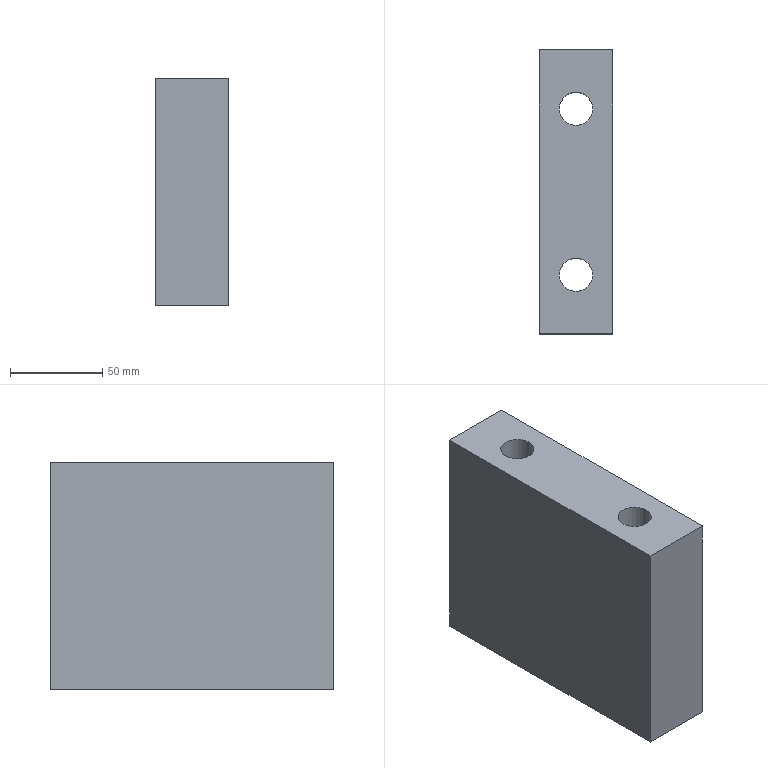Part | NX | features LIN_SOLID_COLOR 2 | 1 solid | 12 faces | box 40 x 154 x 123.5 mm | volume 638424 mm3 | plane 8 | cylinder 4 | commonest cylinder face diameters 18 x2 27 x2
STEP:
#1=CARTESIAN_POINT('',(716.,-77.,-106.5));
#2=VERTEX_POINT('',#1);
#3=CARTESIAN_POINT('',(676.,-77.,-106.5));
#4=VERTEX_POINT('',#3);
#5=CARTESIAN_POINT('',(676.,-77.,-106.5));
#6=DIRECTION('',(-1.,0.,0.));
#7=VECTOR('',#6,1000.);
#8=LINE('',#5,#7);
#9=EDGE_CURVE('',#2,#4,#8,.T.);
#10=ORIENTED_EDGE('',*,*,#9,.T.);
#11=CARTESIAN_POINT('',(676.,-77.,-230.));
#12=VERTEX_POINT('',#11);
#13=CARTESIAN_POINT('',(676.,-77.,-101.5));
#14=DIRECTION('',(0.,0.,1.));
#15=VECTOR('',#14,1000.);
#16=LINE('',#13,#15);
#17=EDGE_CURVE('',#12,#4,#16,.T.);
#18=ORIENTED_EDGE('',*,*,#17,.F.);
#19=CARTESIAN_POINT('',(716.,-77.,-230.));
#20=VERTEX_POINT('',#19);
#21=CARTESIAN_POINT('',(426.,-77.,-230.));
#22=DIRECTION('',(-1.,0.,0.));
#23=VECTOR('',#22,1000.);
#24=LINE('',#21,#23);
#25=EDGE_CURVE('',#20,#12,#24,.T.);
#26=ORIENTED_EDGE('',*,*,#25,.F.);
#27=CARTESIAN_POINT('',(716.,-77.,-101.5));
#28=DIRECTION('',(0.,0.,1.));
#29=VECTOR('',#28,1000.);
#30=LINE('',#27,#29);
#31=EDGE_CURVE('',#20,#2,#30,.T.);
#32=ORIENTED_EDGE('',*,*,#31,.T.);
#33=EDGE_LOOP('',(#10,#18,#26,#32));
#34=FACE_BOUND('',#33,.T.);
#35=CARTESIAN_POINT('',(676.,-77.,-101.5));
#36=DIRECTION('',(0.,1.,0.));
#37=DIRECTION('',(0.,0.,1.));
#38=AXIS2_PLACEMENT_3D('',#35,#36,#37);
#39=PLANE('',#38);
#40=ADVANCED_FACE('',(#34),#39,.F.);
#41=CARTESIAN_POINT('',(676.,77.,-106.5));
#42=VERTEX_POINT('',#41);
#43=CARTESIAN_POINT('',(676.,-160.,-106.5));
#44=DIRECTION('',(0.,-1.,0.));
#45=VECTOR('',#44,1000.);
#46=LINE('',#43,#45);
#47=EDGE_CURVE('',#42,#4,#46,.T.);
#48=ORIENTED_EDGE('',*,*,#47,.F.);
#49=CARTESIAN_POINT('',(676.,77.,-230.));
#50=VERTEX_POINT('',#49);
#51=CARTESIAN_POINT('',(676.,77.,-101.5));
#52=DIRECTION('',(0.,0.,-1.));
#53=VECTOR('',#52,1000.);
#54=LINE('',#51,#53);
#55=EDGE_CURVE('',#50,#42,#54,.F.);
#56=ORIENTED_EDGE('',*,*,#55,.F.);
#57=CARTESIAN_POINT('',(676.,0.,-230.));
#58=DIRECTION('',(0.,1.,0.));
#59=VECTOR('',#58,1000.);
#60=LINE('',#57,#59);
#61=EDGE_CURVE('',#12,#50,#60,.T.);
#62=ORIENTED_EDGE('',*,*,#61,.F.);
#63=ORIENTED_EDGE('',*,*,#17,.T.);
#64=EDGE_LOOP('',(#48,#56,#62,#63));
#65=FACE_BOUND('',#64,.T.);
#66=CARTESIAN_POINT('',(676.,-160.,-101.5));
#67=DIRECTION('',(1.,0.,0.));
#68=DIRECTION('',(0.,0.,1.));
#69=AXIS2_PLACEMENT_3D('',#66,#67,#68);
#70=PLANE('',#69);
#71=ADVANCED_FACE('',(#65),#70,.F.);
#72=CARTESIAN_POINT('',(716.,77.,-230.));
#73=VERTEX_POINT('',#72);
#74=CARTESIAN_POINT('',(716.,77.,-106.5));
#75=VERTEX_POINT('',#74);
#76=CARTESIAN_POINT('',(716.,77.,-101.5));
#77=DIRECTION('',(0.,0.,-1.));
#78=VECTOR('',#77,1000.);
#79=LINE('',#76,#78);
#80=EDGE_CURVE('',#73,#75,#79,.F.);
#81=ORIENTED_EDGE('',*,*,#80,.T.);
#82=CARTESIAN_POINT('',(716.,-160.,-106.5));
#83=DIRECTION('',(0.,-1.,0.));
#84=VECTOR('',#83,1000.);
#85=LINE('',#82,#84);
#86=EDGE_CURVE('',#75,#2,#85,.T.);
#87=ORIENTED_EDGE('',*,*,#86,.T.);
#88=ORIENTED_EDGE('',*,*,#31,.F.);
#89=CARTESIAN_POINT('',(716.,0.,-230.));
#90=DIRECTION('',(0.,1.,0.));
#91=VECTOR('',#90,1000.);
#92=LINE('',#89,#91);
#93=EDGE_CURVE('',#20,#73,#92,.T.);
#94=ORIENTED_EDGE('',*,*,#93,.T.);
#95=EDGE_LOOP('',(#81,#87,#88,#94));
#96=FACE_BOUND('',#95,.T.);
#97=CARTESIAN_POINT('',(716.,-160.,-101.5));
#98=DIRECTION('',(1.,0.,0.));
#99=DIRECTION('',(0.,0.,1.));
#100=AXIS2_PLACEMENT_3D('',#97,#98,#99);
#101=PLANE('',#100);
#102=ADVANCED_FACE('',(#96),#101,.T.);
#103=CARTESIAN_POINT('',(709.5,45.,-230.));
#104=VERTEX_POINT('',#103);
#105=CARTESIAN_POINT('',(696.,45.,-230.));
#106=DIRECTION('',(0.,0.,1.));
#107=DIRECTION('',(1.,0.,0.));
#108=AXIS2_PLACEMENT_3D('',#105,#106,#107);
#109=CIRCLE('',#108,13.5);
#110=EDGE_CURVE('',#104,#104,#109,.T.);
#111=ORIENTED_EDGE('',*,*,#110,.T.);
#112=EDGE_LOOP('',(#111));
#113=FACE_BOUND('',#112,.T.);
#114=CARTESIAN_POINT('',(709.5,-45.,-230.));
#115=VERTEX_POINT('',#114);
#116=CARTESIAN_POINT('',(696.,-45.,-230.));
#117=DIRECTION('',(0.,0.,1.));
#118=DIRECTION('',(1.,0.,0.));
#119=AXIS2_PLACEMENT_3D('',#116,#117,#118);
#120=CIRCLE('',#119,13.5);
#121=EDGE_CURVE('',#115,#115,#120,.T.);
#122=ORIENTED_EDGE('',*,*,#121,.T.);
#123=EDGE_LOOP('',(#122));
#124=FACE_BOUND('',#123,.T.);
#125=ORIENTED_EDGE('',*,*,#61,.T.);
#126=CARTESIAN_POINT('',(676.,77.,-230.));
#127=DIRECTION('',(1.,0.,0.));
#128=VECTOR('',#127,1000.);
#129=LINE('',#126,#128);
#130=EDGE_CURVE('',#73,#50,#129,.F.);
#131=ORIENTED_EDGE('',*,*,#130,.F.);
#132=ORIENTED_EDGE('',*,*,#93,.F.);
#133=ORIENTED_EDGE('',*,*,#25,.T.);
#134=EDGE_LOOP('',(#125,#131,#132,#133));
#135=FACE_BOUND('',#134,.T.);
#136=CARTESIAN_POINT('',(426.,0.,-230.));
#137=DIRECTION('',(0.,0.,1.));
#138=DIRECTION('',(-1.,0.,0.));
#139=AXIS2_PLACEMENT_3D('',#136,#137,#138);
#140=PLANE('',#139);
#141=ADVANCED_FACE('',(#113,#124,#135),#140,.F.);
#142=CARTESIAN_POINT('',(705.,45.,-106.5));
#143=VERTEX_POINT('',#142);
#144=CARTESIAN_POINT('',(696.,45.,-106.5));
#145=DIRECTION('',(0.,0.,-1.));
#146=DIRECTION('',(1.,0.,0.));
#147=AXIS2_PLACEMENT_3D('',#144,#145,#146);
#148=CIRCLE('',#147,9.);
#149=EDGE_CURVE('',#143,#143,#148,.T.);
#150=ORIENTED_EDGE('',*,*,#149,.T.);
#151=EDGE_LOOP('',(#150));
#152=FACE_BOUND('',#151,.T.);
#153=CARTESIAN_POINT('',(705.,-45.,-106.5));
#154=VERTEX_POINT('',#153);
#155=CARTESIAN_POINT('',(696.,-45.,-106.5));
#156=DIRECTION('',(0.,0.,-1.));
#157=DIRECTION('',(1.,0.,0.));
#158=AXIS2_PLACEMENT_3D('',#155,#156,#157);
#159=CIRCLE('',#158,9.);
#160=EDGE_CURVE('',#154,#154,#159,.T.);
#161=ORIENTED_EDGE('',*,*,#160,.T.);
#162=EDGE_LOOP('',(#161));
#163=FACE_BOUND('',#162,.T.);
#164=CARTESIAN_POINT('',(-54.,77.,-106.5));
#165=DIRECTION('',(1.,0.,0.));
#166=VECTOR('',#165,1000.);
#167=LINE('',#164,#166);
#168=EDGE_CURVE('',#75,#42,#167,.F.);
#169=ORIENTED_EDGE('',*,*,#168,.T.);
#170=ORIENTED_EDGE('',*,*,#47,.T.);
#171=ORIENTED_EDGE('',*,*,#9,.F.);
#172=ORIENTED_EDGE('',*,*,#86,.F.);
#173=EDGE_LOOP('',(#169,#170,#171,#172));
#174=FACE_BOUND('',#173,.T.);
#175=CARTESIAN_POINT('',(-54.,-160.,-106.5));
#176=DIRECTION('',(0.,0.,-1.));
#177=DIRECTION('',(1.,0.,0.));
#178=AXIS2_PLACEMENT_3D('',#175,#176,#177);
#179=PLANE('',#178);
#180=ADVANCED_FACE('',(#152,#163,#174),#179,.F.);
#181=ORIENTED_EDGE('',*,*,#130,.T.);
#182=ORIENTED_EDGE('',*,*,#55,.T.);
#183=ORIENTED_EDGE('',*,*,#168,.F.);
#184=ORIENTED_EDGE('',*,*,#80,.F.);
#185=EDGE_LOOP('',(#181,#182,#183,#184));
#186=FACE_BOUND('',#185,.T.);
#187=CARTESIAN_POINT('',(676.,77.,-101.5));
#188=DIRECTION('',(0.,1.,0.));
#189=DIRECTION('',(0.,0.,1.));
#190=AXIS2_PLACEMENT_3D('',#187,#188,#189);
#191=PLANE('',#190);
#192=ADVANCED_FACE('',(#186),#191,.T.);
#193=CARTESIAN_POINT('',(705.,-45.,-136.5));
#194=VERTEX_POINT('',#193);
#195=CARTESIAN_POINT('',(696.,-45.,-136.5));
#196=DIRECTION('',(0.,0.,1.));
#197=DIRECTION('',(1.,0.,0.));
#198=AXIS2_PLACEMENT_3D('',#195,#196,#197);
#199=CIRCLE('',#198,9.);
#200=EDGE_CURVE('',#194,#194,#199,.T.);
#201=ORIENTED_EDGE('',*,*,#200,.F.);
#202=EDGE_LOOP('',(#201));
#203=FACE_BOUND('',#202,.T.);
#204=ORIENTED_EDGE('',*,*,#160,.F.);
#205=EDGE_LOOP('',(#204));
#206=FACE_BOUND('',#205,.T.);
#207=CARTESIAN_POINT('',(696.,-45.,-190.));
#208=DIRECTION('',(0.,0.,1.));
#209=DIRECTION('',(1.,0.,0.));
#210=AXIS2_PLACEMENT_3D('',#207,#208,#209);
#211=CYLINDRICAL_SURFACE('',#210,9.);
#212=ADVANCED_FACE('',(#203,#206),#211,.F.);
#213=ORIENTED_EDGE('',*,*,#200,.T.);
#214=EDGE_LOOP('',(#213));
#215=FACE_BOUND('',#214,.T.);
#216=CARTESIAN_POINT('',(709.5,-45.,-136.5));
#217=VERTEX_POINT('',#216);
#218=CARTESIAN_POINT('',(696.,-45.,-136.5));
#219=DIRECTION('',(0.,0.,-1.));
#220=DIRECTION('',(1.,0.,0.));
#221=AXIS2_PLACEMENT_3D('',#218,#219,#220);
#222=CIRCLE('',#221,13.5);
#223=EDGE_CURVE('',#217,#217,#222,.F.);
#224=ORIENTED_EDGE('',*,*,#223,.F.);
#225=EDGE_LOOP('',(#224));
#226=FACE_BOUND('',#225,.T.);
#227=CARTESIAN_POINT('',(696.,-45.,-136.5));
#228=DIRECTION('',(0.,0.,1.));
#229=DIRECTION('',(1.,0.,0.));
#230=AXIS2_PLACEMENT_3D('',#227,#228,#229);
#231=PLANE('',#230);
#232=ADVANCED_FACE('',(#215,#226),#231,.F.);
#233=ORIENTED_EDGE('',*,*,#223,.T.);
#234=EDGE_LOOP('',(#233));
#235=FACE_BOUND('',#234,.T.);
#236=ORIENTED_EDGE('',*,*,#121,.F.);
#237=EDGE_LOOP('',(#236));
#238=FACE_BOUND('',#237,.T.);
#239=CARTESIAN_POINT('',(696.,-45.,-190.));
#240=DIRECTION('',(0.,0.,1.));
#241=DIRECTION('',(1.,0.,0.));
#242=AXIS2_PLACEMENT_3D('',#239,#240,#241);
#243=CYLINDRICAL_SURFACE('',#242,13.5);
#244=ADVANCED_FACE('',(#235,#238),#243,.F.);
#245=CARTESIAN_POINT('',(705.,45.,-136.5));
#246=VERTEX_POINT('',#245);
#247=CARTESIAN_POINT('',(696.,45.,-136.5));
#248=DIRECTION('',(0.,0.,1.));
#249=DIRECTION('',(1.,0.,0.));
#250=AXIS2_PLACEMENT_3D('',#247,#248,#249);
#251=CIRCLE('',#250,9.);
#252=EDGE_CURVE('',#246,#246,#251,.T.);
#253=ORIENTED_EDGE('',*,*,#252,.F.);
#254=EDGE_LOOP('',(#253));
#255=FACE_BOUND('',#254,.T.);
#256=ORIENTED_EDGE('',*,*,#149,.F.);
#257=EDGE_LOOP('',(#256));
#258=FACE_BOUND('',#257,.T.);
#259=CARTESIAN_POINT('',(696.,45.,-190.));
#260=DIRECTION('',(0.,0.,1.));
#261=DIRECTION('',(1.,0.,0.));
#262=AXIS2_PLACEMENT_3D('',#259,#260,#261);
#263=CYLINDRICAL_SURFACE('',#262,9.);
#264=ADVANCED_FACE('',(#255,#258),#263,.F.);
#265=ORIENTED_EDGE('',*,*,#252,.T.);
#266=EDGE_LOOP('',(#265));
#267=FACE_BOUND('',#266,.T.);
#268=CARTESIAN_POINT('',(709.5,45.,-136.5));
#269=VERTEX_POINT('',#268);
#270=CARTESIAN_POINT('',(696.,45.,-136.5));
#271=DIRECTION('',(0.,0.,1.));
#272=DIRECTION('',(1.,0.,0.));
#273=AXIS2_PLACEMENT_3D('',#270,#271,#272);
#274=CIRCLE('',#273,13.5);
#275=EDGE_CURVE('',#269,#269,#274,.T.);
#276=ORIENTED_EDGE('',*,*,#275,.F.);
#277=EDGE_LOOP('',(#276));
#278=FACE_BOUND('',#277,.T.);
#279=CARTESIAN_POINT('',(696.,-65.,-136.5));
#280=DIRECTION('',(0.,0.,1.));
#281=DIRECTION('',(1.,0.,0.));
#282=AXIS2_PLACEMENT_3D('',#279,#280,#281);
#283=PLANE('',#282);
#284=ADVANCED_FACE('',(#267,#278),#283,.F.);
#285=ORIENTED_EDGE('',*,*,#275,.T.);
#286=EDGE_LOOP('',(#285));
#287=FACE_BOUND('',#286,.T.);
#288=ORIENTED_EDGE('',*,*,#110,.F.);
#289=EDGE_LOOP('',(#288));
#290=FACE_BOUND('',#289,.T.);
#291=CARTESIAN_POINT('',(696.,45.,-190.));
#292=DIRECTION('',(0.,0.,1.));
#293=DIRECTION('',(1.,0.,0.));
#294=AXIS2_PLACEMENT_3D('',#291,#292,#293);
#295=CYLINDRICAL_SURFACE('',#294,13.5);
#296=ADVANCED_FACE('',(#287,#290),#295,.F.);
#297=CLOSED_SHELL('',(#40,#71,#102,#141,#180,#192,#212,#232,#244,#264,#284,#296));
#298=MANIFOLD_SOLID_BREP('',#297);
#299=(LENGTH_UNIT()NAMED_UNIT(*)SI_UNIT(.MILLI.,.METRE.));
#300=UNCERTAINTY_MEASURE_WITH_UNIT(LENGTH_MEASURE(0.00001),#299,'','');
#301=(NAMED_UNIT(*)PLANE_ANGLE_UNIT()SI_UNIT($,.RADIAN.));
#302=(NAMED_UNIT(*)SI_UNIT($,.STERADIAN.)SOLID_ANGLE_UNIT());
#303=(GEOMETRIC_REPRESENTATION_CONTEXT(3)GLOBAL_UNCERTAINTY_ASSIGNED_CONTEXT((#300))GLOBAL_UNIT_ASSIGNED_CONTEXT((#299,#301,#302))REPRESENTATION_CONTEXT('',''));
#304=ADVANCED_BREP_SHAPE_REPRESENTATION('',(#298),#303);